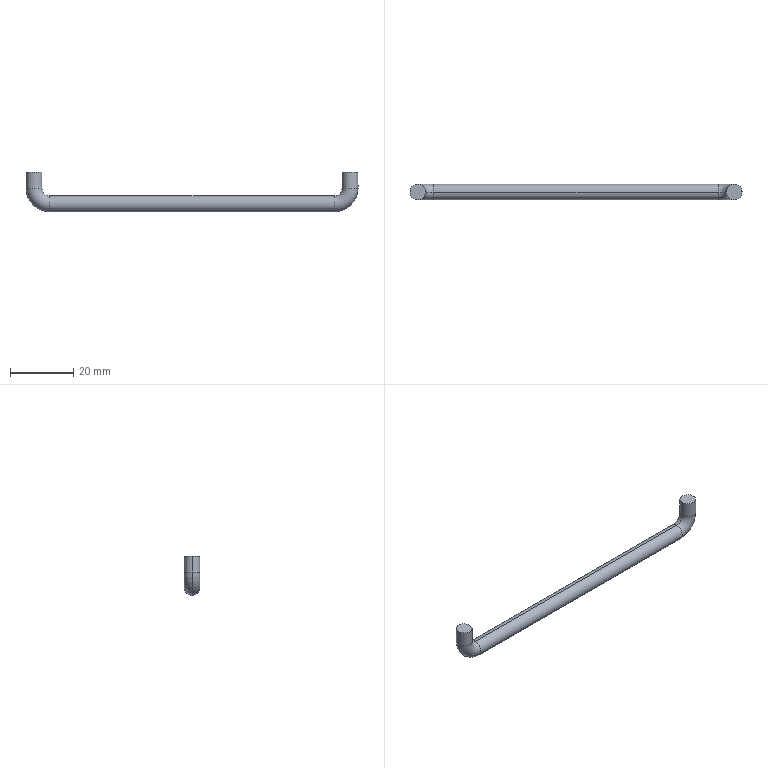Part | SolidWorks | features Sweep 1 | 1 solid | 12 faces | box 105 x 5 x 12.5 mm | volume 2272 mm3 | cylinder 6 | torus 4 | plane 2 | commonest cylinder face diameters 5 x6
STEP:
#1=CARTESIAN_POINT('',(95.,0.,-2.5));
#2=VERTEX_POINT('',#1);
#3=CARTESIAN_POINT('',(95.,0.,2.5));
#4=VERTEX_POINT('',#3);
#5=CARTESIAN_POINT('',(95.,0.,0.));
#6=DIRECTION('',(-1.,0.,0.));
#7=DIRECTION('',(0.,0.,1.));
#8=AXIS2_PLACEMENT_3D('',#5,#6,#7);
#9=CIRCLE('',#8,2.5);
#10=EDGE_CURVE('',#2,#4,#9,.T.);
#11=ORIENTED_EDGE('',*,*,#10,.F.);
#12=CARTESIAN_POINT('',(102.5,0.,5.));
#13=VERTEX_POINT('',#12);
#14=CARTESIAN_POINT('',(95.,0.,5.));
#15=DIRECTION('',(0.,-1.,0.));
#16=DIRECTION('',(0.,0.,-1.));
#17=AXIS2_PLACEMENT_3D('',#14,#15,#16);
#18=CIRCLE('',#17,7.5);
#19=EDGE_CURVE('',#2,#13,#18,.T.);
#20=ORIENTED_EDGE('',*,*,#19,.T.);
#21=CARTESIAN_POINT('',(97.5,0.,5.));
#22=VERTEX_POINT('',#21);
#23=CARTESIAN_POINT('',(100.,0.,5.));
#24=DIRECTION('',(0.,0.,-1.));
#25=DIRECTION('',(-1.,0.,0.));
#26=AXIS2_PLACEMENT_3D('',#23,#24,#25);
#27=CIRCLE('',#26,2.5);
#28=EDGE_CURVE('',#13,#22,#27,.T.);
#29=ORIENTED_EDGE('',*,*,#28,.T.);
#30=CARTESIAN_POINT('',(95.,0.,5.));
#31=DIRECTION('',(0.,-1.,0.));
#32=DIRECTION('',(0.,0.,-1.));
#33=AXIS2_PLACEMENT_3D('',#30,#31,#32);
#34=CIRCLE('',#33,2.5);
#35=EDGE_CURVE('',#4,#22,#34,.T.);
#36=ORIENTED_EDGE('',*,*,#35,.F.);
#37=EDGE_LOOP('',(#11,#20,#29,#36));
#38=FACE_OUTER_BOUND('',#37,.T.);
#39=CARTESIAN_POINT('',(95.,0.,5.));
#40=DIRECTION('',(0.,-1.,0.));
#41=DIRECTION('',(0.,0.,-1.));
#42=AXIS2_PLACEMENT_3D('',#39,#40,#41);
#43=TOROIDAL_SURFACE('',#42,5.,2.5);
#44=ADVANCED_FACE('',(#38),#43,.T.);
#45=CARTESIAN_POINT('',(-2.5,0.,5.));
#46=VERTEX_POINT('',#45);
#47=CARTESIAN_POINT('',(2.5,0.,5.));
#48=VERTEX_POINT('',#47);
#49=CARTESIAN_POINT('',(0.,0.,5.));
#50=DIRECTION('',(0.,0.,1.));
#51=DIRECTION('',(1.,0.,0.));
#52=AXIS2_PLACEMENT_3D('',#49,#50,#51);
#53=CIRCLE('',#52,2.5);
#54=EDGE_CURVE('',#46,#48,#53,.T.);
#55=ORIENTED_EDGE('',*,*,#54,.F.);
#56=CARTESIAN_POINT('',(5.,0.,-2.5));
#57=VERTEX_POINT('',#56);
#58=CARTESIAN_POINT('',(5.,0.,5.));
#59=DIRECTION('',(0.,-1.,0.));
#60=DIRECTION('',(0.,0.,-1.));
#61=AXIS2_PLACEMENT_3D('',#58,#59,#60);
#62=CIRCLE('',#61,7.5);
#63=EDGE_CURVE('',#46,#57,#62,.T.);
#64=ORIENTED_EDGE('',*,*,#63,.T.);
#65=CARTESIAN_POINT('',(5.,0.,2.5));
#66=VERTEX_POINT('',#65);
#67=CARTESIAN_POINT('',(5.,0.,0.));
#68=DIRECTION('',(-1.,0.,0.));
#69=DIRECTION('',(0.,0.,1.));
#70=AXIS2_PLACEMENT_3D('',#67,#68,#69);
#71=CIRCLE('',#70,2.5);
#72=EDGE_CURVE('',#57,#66,#71,.T.);
#73=ORIENTED_EDGE('',*,*,#72,.T.);
#74=CARTESIAN_POINT('',(5.,0.,5.));
#75=DIRECTION('',(0.,-1.,0.));
#76=DIRECTION('',(0.,0.,-1.));
#77=AXIS2_PLACEMENT_3D('',#74,#75,#76);
#78=CIRCLE('',#77,2.5);
#79=EDGE_CURVE('',#48,#66,#78,.T.);
#80=ORIENTED_EDGE('',*,*,#79,.F.);
#81=EDGE_LOOP('',(#55,#64,#73,#80));
#82=FACE_OUTER_BOUND('',#81,.T.);
#83=CARTESIAN_POINT('',(5.,0.,5.));
#84=DIRECTION('',(0.,-1.,0.));
#85=DIRECTION('',(0.,0.,-1.));
#86=AXIS2_PLACEMENT_3D('',#83,#84,#85);
#87=TOROIDAL_SURFACE('',#86,5.,2.5);
#88=ADVANCED_FACE('',(#82),#87,.T.);
#89=CARTESIAN_POINT('',(100.,0.,5.));
#90=DIRECTION('',(0.,0.,-1.));
#91=DIRECTION('',(-1.,0.,0.));
#92=AXIS2_PLACEMENT_3D('',#89,#90,#91);
#93=CIRCLE('',#92,2.5);
#94=EDGE_CURVE('',#22,#13,#93,.T.);
#95=ORIENTED_EDGE('',*,*,#94,.F.);
#96=CARTESIAN_POINT('',(97.5,0.,10.));
#97=VERTEX_POINT('',#96);
#98=CARTESIAN_POINT('',(97.5,0.,5.));
#99=DIRECTION('',(0.,0.,1.));
#100=VECTOR('',#99,1000.);
#101=LINE('',#98,#100);
#102=EDGE_CURVE('',#22,#97,#101,.T.);
#103=ORIENTED_EDGE('',*,*,#102,.T.);
#104=CARTESIAN_POINT('',(102.5,0.,10.));
#105=VERTEX_POINT('',#104);
#106=CARTESIAN_POINT('',(100.,0.,10.));
#107=DIRECTION('',(0.,0.,-1.));
#108=DIRECTION('',(-1.,0.,0.));
#109=AXIS2_PLACEMENT_3D('',#106,#107,#108);
#110=CIRCLE('',#109,2.5);
#111=EDGE_CURVE('',#97,#105,#110,.T.);
#112=ORIENTED_EDGE('',*,*,#111,.T.);
#113=CARTESIAN_POINT('',(102.5,0.,5.));
#114=DIRECTION('',(0.,0.,1.));
#115=VECTOR('',#114,1000.);
#116=LINE('',#113,#115);
#117=EDGE_CURVE('',#13,#105,#116,.T.);
#118=ORIENTED_EDGE('',*,*,#117,.F.);
#119=EDGE_LOOP('',(#95,#103,#112,#118));
#120=FACE_OUTER_BOUND('',#119,.T.);
#121=CARTESIAN_POINT('',(100.,0.,5.));
#122=DIRECTION('',(0.,0.,1.));
#123=DIRECTION('',(1.,0.,0.));
#124=AXIS2_PLACEMENT_3D('',#121,#122,#123);
#125=CYLINDRICAL_SURFACE('',#124,2.5);
#126=ADVANCED_FACE('',(#120),#125,.T.);
#127=CARTESIAN_POINT('',(5.,0.,0.));
#128=DIRECTION('',(-1.,0.,0.));
#129=DIRECTION('',(0.,0.,1.));
#130=AXIS2_PLACEMENT_3D('',#127,#128,#129);
#131=CIRCLE('',#130,2.5);
#132=EDGE_CURVE('',#66,#57,#131,.T.);
#133=ORIENTED_EDGE('',*,*,#132,.F.);
#134=CARTESIAN_POINT('',(5.,0.,2.5));
#135=DIRECTION('',(1.,0.,0.));
#136=VECTOR('',#135,1000.);
#137=LINE('',#134,#136);
#138=EDGE_CURVE('',#66,#4,#137,.T.);
#139=ORIENTED_EDGE('',*,*,#138,.T.);
#140=CARTESIAN_POINT('',(95.,0.,0.));
#141=DIRECTION('',(-1.,0.,0.));
#142=DIRECTION('',(0.,0.,1.));
#143=AXIS2_PLACEMENT_3D('',#140,#141,#142);
#144=CIRCLE('',#143,2.5);
#145=EDGE_CURVE('',#4,#2,#144,.T.);
#146=ORIENTED_EDGE('',*,*,#145,.T.);
#147=CARTESIAN_POINT('',(5.,0.,-2.5));
#148=DIRECTION('',(1.,0.,0.));
#149=VECTOR('',#148,1000.);
#150=LINE('',#147,#149);
#151=EDGE_CURVE('',#57,#2,#150,.T.);
#152=ORIENTED_EDGE('',*,*,#151,.F.);
#153=EDGE_LOOP('',(#133,#139,#146,#152));
#154=FACE_OUTER_BOUND('',#153,.T.);
#155=CARTESIAN_POINT('',(5.,0.,0.));
#156=DIRECTION('',(1.,0.,0.));
#157=DIRECTION('',(0.,0.,-1.));
#158=AXIS2_PLACEMENT_3D('',#155,#156,#157);
#159=CYLINDRICAL_SURFACE('',#158,2.5);
#160=ADVANCED_FACE('',(#154),#159,.T.);
#161=CARTESIAN_POINT('',(2.5,0.,10.));
#162=VERTEX_POINT('',#161);
#163=CARTESIAN_POINT('',(-2.5,0.,10.));
#164=VERTEX_POINT('',#163);
#165=CARTESIAN_POINT('',(0.,0.,10.));
#166=DIRECTION('',(0.,0.,1.));
#167=DIRECTION('',(1.,0.,0.));
#168=AXIS2_PLACEMENT_3D('',#165,#166,#167);
#169=CIRCLE('',#168,2.5);
#170=EDGE_CURVE('',#162,#164,#169,.T.);
#171=ORIENTED_EDGE('',*,*,#170,.F.);
#172=CARTESIAN_POINT('',(2.5,0.,10.));
#173=DIRECTION('',(0.,0.,-1.));
#174=VECTOR('',#173,1000.);
#175=LINE('',#172,#174);
#176=EDGE_CURVE('',#162,#48,#175,.T.);
#177=ORIENTED_EDGE('',*,*,#176,.T.);
#178=CARTESIAN_POINT('',(0.,0.,5.));
#179=DIRECTION('',(0.,0.,1.));
#180=DIRECTION('',(1.,0.,0.));
#181=AXIS2_PLACEMENT_3D('',#178,#179,#180);
#182=CIRCLE('',#181,2.5);
#183=EDGE_CURVE('',#48,#46,#182,.T.);
#184=ORIENTED_EDGE('',*,*,#183,.T.);
#185=CARTESIAN_POINT('',(-2.5,0.,10.));
#186=DIRECTION('',(0.,0.,-1.));
#187=VECTOR('',#186,1000.);
#188=LINE('',#185,#187);
#189=EDGE_CURVE('',#164,#46,#188,.T.);
#190=ORIENTED_EDGE('',*,*,#189,.F.);
#191=EDGE_LOOP('',(#171,#177,#184,#190));
#192=FACE_OUTER_BOUND('',#191,.T.);
#193=CARTESIAN_POINT('',(0.,0.,10.));
#194=DIRECTION('',(0.,0.,-1.));
#195=DIRECTION('',(-1.,0.,0.));
#196=AXIS2_PLACEMENT_3D('',#193,#194,#195);
#197=CYLINDRICAL_SURFACE('',#196,2.5);
#198=ADVANCED_FACE('',(#192),#197,.T.);
#199=ORIENTED_EDGE('',*,*,#102,.F.);
#200=ORIENTED_EDGE('',*,*,#28,.F.);
#201=ORIENTED_EDGE('',*,*,#117,.T.);
#202=CARTESIAN_POINT('',(100.,0.,10.));
#203=DIRECTION('',(0.,0.,-1.));
#204=DIRECTION('',(-1.,0.,0.));
#205=AXIS2_PLACEMENT_3D('',#202,#203,#204);
#206=CIRCLE('',#205,2.5);
#207=EDGE_CURVE('',#105,#97,#206,.T.);
#208=ORIENTED_EDGE('',*,*,#207,.T.);
#209=EDGE_LOOP('',(#199,#200,#201,#208));
#210=FACE_OUTER_BOUND('',#209,.T.);
#211=CARTESIAN_POINT('',(100.,0.,5.));
#212=DIRECTION('',(0.,0.,1.));
#213=DIRECTION('',(1.,0.,0.));
#214=AXIS2_PLACEMENT_3D('',#211,#212,#213);
#215=CYLINDRICAL_SURFACE('',#214,2.5);
#216=ADVANCED_FACE('',(#210),#215,.T.);
#217=ORIENTED_EDGE('',*,*,#19,.F.);
#218=ORIENTED_EDGE('',*,*,#145,.F.);
#219=ORIENTED_EDGE('',*,*,#35,.T.);
#220=ORIENTED_EDGE('',*,*,#94,.T.);
#221=EDGE_LOOP('',(#217,#218,#219,#220));
#222=FACE_OUTER_BOUND('',#221,.T.);
#223=CARTESIAN_POINT('',(95.,0.,5.));
#224=DIRECTION('',(0.,-1.,0.));
#225=DIRECTION('',(0.,0.,-1.));
#226=AXIS2_PLACEMENT_3D('',#223,#224,#225);
#227=TOROIDAL_SURFACE('',#226,5.,2.5);
#228=ADVANCED_FACE('',(#222),#227,.T.);
#229=ORIENTED_EDGE('',*,*,#138,.F.);
#230=ORIENTED_EDGE('',*,*,#72,.F.);
#231=ORIENTED_EDGE('',*,*,#151,.T.);
#232=ORIENTED_EDGE('',*,*,#10,.T.);
#233=EDGE_LOOP('',(#229,#230,#231,#232));
#234=FACE_OUTER_BOUND('',#233,.T.);
#235=CARTESIAN_POINT('',(5.,0.,0.));
#236=DIRECTION('',(1.,0.,0.));
#237=DIRECTION('',(0.,0.,-1.));
#238=AXIS2_PLACEMENT_3D('',#235,#236,#237);
#239=CYLINDRICAL_SURFACE('',#238,2.5);
#240=ADVANCED_FACE('',(#234),#239,.T.);
#241=ORIENTED_EDGE('',*,*,#63,.F.);
#242=ORIENTED_EDGE('',*,*,#183,.F.);
#243=ORIENTED_EDGE('',*,*,#79,.T.);
#244=ORIENTED_EDGE('',*,*,#132,.T.);
#245=EDGE_LOOP('',(#241,#242,#243,#244));
#246=FACE_OUTER_BOUND('',#245,.T.);
#247=CARTESIAN_POINT('',(5.,0.,5.));
#248=DIRECTION('',(0.,-1.,0.));
#249=DIRECTION('',(0.,0.,-1.));
#250=AXIS2_PLACEMENT_3D('',#247,#248,#249);
#251=TOROIDAL_SURFACE('',#250,5.,2.5);
#252=ADVANCED_FACE('',(#246),#251,.T.);
#253=ORIENTED_EDGE('',*,*,#176,.F.);
#254=CARTESIAN_POINT('',(0.,0.,10.));
#255=DIRECTION('',(0.,0.,1.));
#256=DIRECTION('',(1.,0.,0.));
#257=AXIS2_PLACEMENT_3D('',#254,#255,#256);
#258=CIRCLE('',#257,2.5);
#259=EDGE_CURVE('',#164,#162,#258,.T.);
#260=ORIENTED_EDGE('',*,*,#259,.F.);
#261=ORIENTED_EDGE('',*,*,#189,.T.);
#262=ORIENTED_EDGE('',*,*,#54,.T.);
#263=EDGE_LOOP('',(#253,#260,#261,#262));
#264=FACE_OUTER_BOUND('',#263,.T.);
#265=CARTESIAN_POINT('',(0.,0.,10.));
#266=DIRECTION('',(0.,0.,-1.));
#267=DIRECTION('',(-1.,0.,0.));
#268=AXIS2_PLACEMENT_3D('',#265,#266,#267);
#269=CYLINDRICAL_SURFACE('',#268,2.5);
#270=ADVANCED_FACE('',(#264),#269,.T.);
#271=ORIENTED_EDGE('',*,*,#207,.F.);
#272=ORIENTED_EDGE('',*,*,#111,.F.);
#273=EDGE_LOOP('',(#271,#272));
#274=FACE_OUTER_BOUND('',#273,.T.);
#275=CARTESIAN_POINT('',(100.,0.,10.));
#276=DIRECTION('',(0.,0.,-1.));
#277=DIRECTION('',(-1.,0.,0.));
#278=AXIS2_PLACEMENT_3D('',#275,#276,#277);
#279=PLANE('',#278);
#280=ADVANCED_FACE('',(#274),#279,.F.);
#281=ORIENTED_EDGE('',*,*,#259,.T.);
#282=ORIENTED_EDGE('',*,*,#170,.T.);
#283=EDGE_LOOP('',(#281,#282));
#284=FACE_OUTER_BOUND('',#283,.T.);
#285=CARTESIAN_POINT('',(0.,0.,10.));
#286=DIRECTION('',(0.,0.,1.));
#287=DIRECTION('',(1.,0.,0.));
#288=AXIS2_PLACEMENT_3D('',#285,#286,#287);
#289=PLANE('',#288);
#290=ADVANCED_FACE('',(#284),#289,.T.);
#291=CLOSED_SHELL('',(#44,#88,#126,#160,#198,#216,#228,#240,#252,#270,#280,#290));
#292=MANIFOLD_SOLID_BREP('',#291);
#293=CARTESIAN_POINT('',(0.,0.,0.));
#294=DIRECTION('',(0.,0.,1.));
#295=DIRECTION('',(1.,0.,0.));
#296=AXIS2_PLACEMENT_3D('',#293,#294,#295);
#297=(LENGTH_UNIT()NAMED_UNIT(*)SI_UNIT(.MILLI.,.METRE.));
#298=UNCERTAINTY_MEASURE_WITH_UNIT(LENGTH_MEASURE(0.00001),#297,'','');
#299=(NAMED_UNIT(*)PLANE_ANGLE_UNIT()SI_UNIT($,.RADIAN.));
#300=(NAMED_UNIT(*)SI_UNIT($,.STERADIAN.)SOLID_ANGLE_UNIT());
#301=(GEOMETRIC_REPRESENTATION_CONTEXT(3)GLOBAL_UNCERTAINTY_ASSIGNED_CONTEXT((#298))GLOBAL_UNIT_ASSIGNED_CONTEXT((#297,#299,#300))REPRESENTATION_CONTEXT('',''));
#302=ADVANCED_BREP_SHAPE_REPRESENTATION('',(#292,#296),#301);